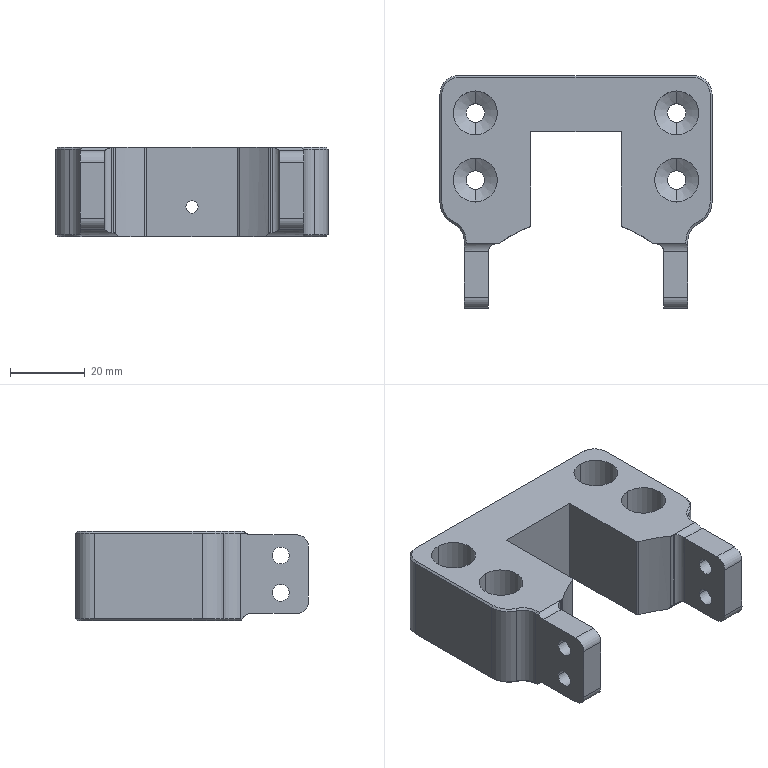NC program | NX | posted with a generic post | part box 73 x 62.4 x 24 mm
Lines 110 to 988 of 11507:
(ADAPTIVE_MILLING , TOOL : D10)
N176 T10 M6
N178 G54
N180 G17 G0 G90 X-47.247 Y-0.01 S8000 M3
N182 G43 Z30. H10
N184 Z-9.
N186 G94 G1 Z-12. F1000.
N188 X-45.053 Y-0.272 F3500.
N190 G3 X-44.622 Y-0.01 R0.536
N192 X-43.825 Y2.911 R7.188
N194 X-43.521 Y11.777 R90.492
N196 G1 X-43.514 Y13.652
N198 X-43.51 Y16.402
N200 X-43.508 Y21.652
N202 X-43.507 Y31.027
N204 X-43.506 Y31.277
N206 X-43.502 Y31.402
N208 G2 X-40.935 Y35.647 R5.829
N210 X-35.479 Y37.674 R12.556
N212 X-27.25 Y38.153 R59.855
N214 G1 X-26.25 Y38.162
N216 X-25.125 Y38.17
N218 X-23.5 Y38.177
N220 X-21.25 Y38.182
N222 X-17.625 Y38.185
N224 X-6. Y38.186
N226 X36.5
N228 X36.625 Y38.184
N230 X36.749 Y38.179
N232 X36.874 Y38.17
N234 G2 X41.05 Y35.485 R5.897
N236 X43.003 Y29.999 R12.841
N238 X43.452 Y22.018 R60.705
N240 G1 X43.463 Y20.893
N242 X43.471 Y19.518
N244 X43.478 Y17.643
N246 X43.482 Y15.268
N248 X43.485 Y10.768
N250 X43.486 Y-26.982
N252 Y-31.232
N254 X43.484 Y-31.357
N256 X43.477 Y-31.482
N258 X43.466 Y-31.606
N260 G2 X40.649 Y-35.837 R6.001
N262 X34.89 Y-37.759 R13.462
N264 X25.655 Y-38.167 R79.348
N266 G1 X24.155 Y-38.175
N268 X22.155 Y-38.18
N270 X19.03 Y-38.184
N272 X12.155 Y-38.186
N274 X-36.47
N276 X-36.595 Y-38.185
N278 G2 X-40.81 Y-35.809 R5.653
N280 X-42.96 Y-30.274 R12.12
N282 X-43.445 Y-22.546 R54.637
N284 X-43.457 Y-2.797 R922.246
N286 G3 X-42.766 Y4.168 R369.786
N288 X-42.523 Y17.914 R254.659
N290 G2 X-42.488 Y28.788 R700.753
N292 X-38.545 Y34.698 R7.841
N294 X-32.028 Y36.72 R16.354
N296 X-22.168 Y37.152 R90.427
N298 G1 X-20.793 Y37.16
N300 X-18.918 Y37.167
N302 X-16.293 Y37.172
N304 X-11.918 Y37.175
N306 X6.457
N308 X33.332
N310 G2 X39.797 Y33.54 R7.602
N312 X41.973 Y27.079 R15.41
N314 X42.447 Y17.472 R79.405
N316 G1 X42.457 Y16.097
N318 X42.464 Y14.472
N320 X42.469 Y12.347
N322 X42.473 Y8.847
N324 X42.475 Y1.097
N326 Y-28.028
N328 G2 X38.842 Y-34.494 R7.602
N330 X32.505 Y-36.656 R15.316
N332 X23.399 Y-37.141 R74.48
N334 G1 X22.274 Y-37.151
N336 X20.899 Y-37.16
N338 X19.274 Y-37.166
N340 X16.899 Y-37.171
N342 X13.024 Y-37.174
N344 X1.649 Y-37.175
N346 X-33.351
N348 X-33.601 Y-37.173
N350 X-33.851 Y-37.164
N352 G2 X-39.875 Y-33.42 R7.671
N354 X-41.991 Y-26.936 R15.797
N356 X-42.451 Y-16.953 R85.053
N358 X-42.428 Y-4.204 R448.54
N360 G3 X-41.769 Y4.771 R957.119
N362 G1 X-41.734 Y5.52
N364 X-41.703 Y6.27
N366 X-41.675 Y7.019
N368 X-41.651 Y7.769
N370 X-41.65 Y7.82
N372 Y26.186
N374 X-41.649 Y26.214
N376 X-41.458 Y28.153
N378 X-41.447 Y28.207
N380 X-40.885 Y30.058
N382 X-40.864 Y30.109
N384 X-39.952 Y31.815
N386 X-39.922 Y31.86
N388 X-38.695 Y33.356
N390 X-38.656 Y33.395
N392 X-37.16 Y34.622
N394 X-37.115 Y34.652
N396 X-35.409 Y35.564
N398 X-35.358 Y35.585
N400 X-33.507 Y36.147
N402 X-33.453 Y36.158
N404 X-31.514 Y36.349
N406 X-31.486 Y36.35
N408 X31.486
N410 X31.514 Y36.349
N412 X33.453 Y36.158
N414 X33.507 Y36.147
N416 X35.358 Y35.585
N418 X35.409 Y35.564
N420 X37.115 Y34.652
N422 X37.16 Y34.622
N424 X38.656 Y33.395
N426 X38.695 Y33.356
N428 X39.922 Y31.86
N430 X39.952 Y31.815
N432 X40.864 Y30.109
N434 X40.885 Y30.058
N436 X41.447 Y28.207
N438 X41.458 Y28.153
N440 X41.649 Y26.214
N442 X41.65 Y26.186
N444 Y-2.689
N446 X41.649 Y-2.711
N448 X41.629 Y-2.96
N450 G3 X41.488 Y-14.458 R298.961
N452 G2 X41.447 Y-26.458 R542.382
N454 X36.69 Y-33.65 R8.945
N456 X33.443 Y-34.995 R16.931
N458 X31.293 Y-36.18 R5.576
N460 G1 X30.018 Y-36.348
N462 X29.982 Y-36.35
N464 G2 X19.734 Y-36.22 R205.958
N466 G1 X18.734 Y-36.209
N468 X17.609 Y-36.201
N470 X16.109 Y-36.194
N472 X13.984 Y-36.189
N474 X10.359 Y-36.187
N476 X-3.516 Y-36.186
N478 X-4.266 Y-36.183
N480 X-5.391 Y-36.181
N482 X-6.266
N484 X-7.015 Y-36.179
N486 X-8.14
N488 X-8.515
N490 X-9.39 Y-36.177
N492 X-10.39 Y-36.178
N494 X-10.89 Y-36.179
N496 X-11.515 Y-36.177
N498 X-12.89 Y-36.178
N500 X-13.64 Y-36.179
N502 X-14.64 Y-36.176
N504 X-15.89 Y-36.178
N506 X-16.64 Y-36.176
N508 X-17.64 Y-36.177
N510 X-18.015 Y-36.178
N512 X-19.265 Y-36.175
N514 X-20.14 Y-36.176
N516 X-21.39 Y-36.174
N518 X-22.192 Y-36.176
N520 X-22.204 Y-36.179
N522 X-23.482 Y-36.348
N524 X-23.518 Y-36.35
N526 G2 X-31.142 Y-36.29 R145.108
N528 X-39.063 Y-31.222 R9.185
N530 X-41.041 Y-24.037 R19.418
N532 X-41.445 Y-13.049 R114.967
N534 X-41.405 Y-4.949 R285.925
N536 X-41.65 Y-2.689 R13.093
N538 G1 Y7.936
N540 G3 X-42.562 Y8.219 R0.5
N542 G1 X-42.912 Y7.71
N544 X-44.043 Y6.06 Z-11.9
N546 X-44.782 Y4.972
N548 X-44.832 Y4.754
N550 X-44.825 Y-16.153
N552 G3 X-44.01 Y-25.178 R60.801
N554 G1 X-43.51 Y-28.132
N556 G3 X-41.324 Y-33.684 R17.035
N558 X-38.292 Y-36.846 R11.782
N560 X-35.905 Y-38.261 R14.75
N562 G1 X-33.127 Y-39.557
N564 G3 X-32.683 Y-39.473 R0.513
N566 G1 X-31.648 Y-38.678
N568 X-30.063 Y-37.458 Z-12.
N570 X-29.852 Y-37.301
N572 X-29.665 Y-37.117
N574 G3 X-30.018 Y-36.348 R0.501
N576 G2 X-33.451 Y-35.106 R6.123
N578 X-39.075 Y-27.253 R13.64
N580 X-40.254 Y-19.107 R34.794
N582 X-40.454 Y-7.801 R296.213
N584 X-41.426 Y-4.863 R11.519
N586 G3 X-42.386 Y-4.822 R0.5
N588 G1 X-42.647 Y-5.603
N590 X-43.281 Y-7.499 Z-11.9
N592 X-43.669 Y-8.68
N594 X-43.679 Y-11.878
N596 X-43.649 Y-15.077
N598 G3 X-43.147 Y-21.853 R73.461
N600 G1 X-42.967 Y-23.333
N602 X-42.761 Y-24.81
N604 G3 X-41.089 Y-30.413 R22.619
N606 X-39.632 Y-33.007 R18.982
N608 X-36.901 Y-36.859 R63.987
N610 X-36.486 Y-36.999 R0.514
N612 G1 X-35.18 Y-36.831
N614 X-33.196 Y-36.575 Z-12.
N616 X-32.937 Y-36.546
N618 X-32.684 Y-36.481
N620 G3 X-32.604 Y-35.638 R0.501
N622 G2 X-34.505 Y-33.699 R5.992
N624 X-38.885 Y-21.875 R24.702
N626 X-39.417 Y-10.143 R111.218
N628 G3 X-39.498 Y-9.417 R5.368
N630 G2 X-40.455 Y-7.797 R15.222
N632 G3 X-41.388 Y-7.826 R0.501
N634 G1 X-41.457 Y-8.023
N636 X-42.117 Y-9.911 Z-11.9
N638 X-42.694 Y-11.573
N640 X-42.705 Y-11.694
N642 X-42.629 Y-14.189
N644 X-42.497 Y-16.681
N646 X-42.383 Y-17.923
N648 X-42.252 Y-19.163
N650 X-41.451 Y-25.67
N652 G3 X-39.988 Y-30.246 R15.486
N654 G1 X-38.741 Y-32.71
N656 X-38.653 Y-32.797
N658 X-38.551 Y-32.867
N660 X-37.31 Y-33.454
N662 X-35.502 Y-34.309 Z-12.
N664 X-35.005 Y-34.536
N666 G3 X-34.438 Y-33.804 R0.501
N668 G2 X-35.363 Y-31.177 R16.109
N670 X-38.205 Y-16.643 R45.398
N672 G3 X-38.447 Y-11.025 R192.609
N674 X-38.582 Y-10.529 R4.593
N676 G2 X-39.516 Y-9.388 R12.129
N678 G3 X-40.523 Y-9.784 R0.55
N680 G1 X-40.331 Y-10.77
N682 X-39.949 Y-12.733 Z-11.9
N684 X-37.652 Y-24.522
N686 X-37.27 Y-26.486 Z-12.
N688 X-36.04 Y-32.759
N690 G3 X-34.979 Y-32.496 R0.55
N692 G2 X-35.274 Y-29.689 R92.746
N694 X-36.6 Y-22.308 R220.445
N696 X-37.332 Y-13.091 R114.757
N698 G3 X-37.621 Y-11.5 R5.66
N700 G2 X-38.584 Y-10.527 R11.27
N702 G3 X-39.541 Y-10.977 R0.55
N704 G1 X-39.46 Y-11.469
N706 X-39.136 Y-13.442 Z-11.9
N708 X-37.651 Y-22.462
N710 X-37.327 Y-24.435 Z-12.
N712 X-36.221 Y-31.109
N714 G3 X-35.15 Y-30.932 R0.55
N716 X-35.615 Y-22.33 R51.445
N718 G2 X-36.317 Y-13.859 R506.421
N720 G3 X-36.68 Y-12.283 R6.352
N722 G1 X-36.755 Y-12.19
N724 X-37.716 Y-11.387
N726 G3 X-38.612 Y-11.892 R0.551
N728 G1 X-36.244 Y-27.39
N730 G3 X-35.15 Y-27.307 R0.55
N732 X-35.19 Y-16.557 R427.104
N734 X-35.739 Y-12.99 R11.724
N736 G1 X-35.962 Y-12.666
N738 X-36.72 Y-12.214
N740 X-36.757 Y-12.188
N742 G3 X-37.605 Y-12.782 R0.551
N744 G1 X-36.201 Y-17.909
N746 G3 X-35.15 Y-17.682 R0.55
N748 X-35.19 Y-13.559 R55.738
N750 X-35.474 Y-12.957 R1.065
N752 G1 X-36.011 Y-12.637
N754 G3 X-36.738 Y-13.431 R0.55
N756 G1 X-36.09 Y-14.319
N758 G3 X-35.15 Y-13.932 R0.551
N760 X-35.278 Y-13.112 R1.289
N762 G1 X-35.425 Y-12.986
N764 X-35.532 Y-12.922
N766 G3 X-36.163 Y-13.021 R0.504
N768 G1 X-36.323 Y-13.203
N770 X-37.646 Y-14.703 Z-11.9
N772 X-38.633 Y-15.831
N774 X-38.69 Y-15.963
N776 X-38.714 Y-16.104
N778 X-38.707 Y-29.055
N780 G3 X-37.508 Y-34.639 R16.449
N782 X-35.731 Y-37.093 R7.053
N784 G1 X-34.606 Y-38.082
N786 G3 X-32.584 Y-38.971 R4.306
N788 X-29.225 Y-39.383 R37.795
N790 G1 X-27.623 Y-39.436
N792 X20.376 Y-39.524
N794 X20.485 Y-39.488
N796 X20.588 Y-39.439
N798 X21.723 Y-38.643
N800 X23.36 Y-37.494 Z-12.
N802 X23.769 Y-37.198
N804 G3 X23.482 Y-36.348 R0.501
N806 G2 X21.308 Y-35.87 R6.827
N808 G3 X15.6 Y-35.283 R27.258
N810 X-4.149 Y-35.186 R984.653
N812 G1 X-5.274 Y-35.184
N814 X-6.149
N816 X-7.149 Y-35.181
N818 X-8.274 Y-35.182
N820 X-9.024 Y-35.18
N822 X-10.149
N824 X-10.774 Y-35.181
N826 X-12.024 Y-35.177
N828 X-13.024 Y-35.179
N830 X-14.149 Y-35.177
N832 X-15.149 Y-35.178
N834 X-16.149 Y-35.176
N836 X-16.899
N838 X-17.649 Y-35.178
N840 X-18.774 Y-35.175
N842 X-19.524 Y-35.176
N844 X-19.649 Y-35.177
N846 X-19.899 Y-35.181
N848 G3 X-20.415 Y-35.269 R1.866
N850 G1 X-20.896 Y-35.638
N852 X-20.959 Y-35.674
N854 X-22.133 Y-36.16
N856 X-22.204 Y-36.179
N858 G3 X-22.06 Y-37.261 R0.55
N860 G1 X-20.92 Y-37.257
N862 X-18.92 Y-37.251 Z-11.9
N864 X18.72 Y-37.132
N866 X20.72 Y-37.126 Z-12.
N868 X21.782 Y-37.115
N870 G3 X21.902 Y-36.065 R0.55
N872 G2 X19.994 Y-35.21 R91.635
N874 G3 X14.574 Y-34.382 R20.379
N876 X-0.673 Y-34.201 R389.778
N878 G1 X-1.423 Y-34.197
N880 X-2.548 Y-34.194
N882 X-3.548 Y-34.193
N884 X-4.423 Y-34.189
N886 X-5.298 Y-34.188
N888 X-6.173 Y-34.186
N890 X-6.798 Y-34.183
N892 X-7.923 Y-34.184
N894 X-8.548 Y-34.182
N896 X-9.173 Y-34.18
N898 X-10.173 Y-34.181
N900 X-11.298 Y-34.178
N902 X-12.548 Y-34.18
N904 X-13.798 Y-34.177
N906 X-14.798 Y-34.179
N908 X-15.798 Y-34.176
N910 G3 X-19.289 Y-34.322 R20.036
N912 X-19.888 Y-34.864 R1.346
N914 G1 X-20.483 Y-35.321
N916 G3 X-20.152 Y-36.307 R0.551
N918 G1 X-19.86 Y-36.309
N920 X-17.86 Y-36.325 Z-11.9
N922 X18.083 Y-36.605
N924 X20.083 Y-36.62 Z-12.
N926 X20.648 Y-36.617
N928 G3 X20.896 Y-35.638 R0.551
N930 X17.074 Y-33.911 R7.517
N932 X9.608 Y-33.3 R45.798
N934 X-12.141 Y-33.18 R985.897
N936 X-17.762 Y-33.296 R58.939
N938 X-18.946 Y-33.652 R2.657
N940 G1 X-19.026 Y-33.741
N942 X-19.062 Y-33.804
N944 X-19.595 Y-34.498
N946 G3 X-19.173 Y-35.383 R0.551
N948 G1 X-17.173 Y-35.416 Z-11.9
N950 X17.573 Y-35.98
N952 X19.572 Y-36.012 Z-12.
N954 G3 X20.082 Y-35.916 R0.788
N956 X20.102 Y-35.029 R0.551
N958 X19.195 Y-34.223 R26.233
N960 X15.075 Y-32.848 R10.727
N962 X6.475 Y-32.29 R63.923
N964 X-15.399 Y-32.225 R858.486
N966 X-18.333 Y-32.75 R7.91
N968 X-18.752 Y-33.08 R1.363
N970 G1 X-19.026 Y-33.741
N972 X-19.062 Y-33.804
N974 G3 X-18.719 Y-34.613 R0.551
N976 G1 X-18.066 Y-34.649 Z-11.967
N978 X-17.413 Y-34.659 Z-11.935
N980 X-16.721 Y-34.677 Z-11.9
N982 X17.237 Y-35.545
N984 X19.236 Y-35.596 Z-12.
N986 G3 X19.76 Y-34.713 R0.555
N988 X16.763 Y-32.587 R5.404
N990 X10.121 Y-31.496 R25.906
N992 X-7.249 Y-31.198 R351.051
N994 X-15.371 Y-31.319 R108.78
N996 X-18.241 Y-32.096 R6.684
N998 X-18.54 Y-32.567 R0.772
N1000 G1 X-18.779 Y-33.144
N1002 G3 X-18.424 Y-33.883 R0.552
N1004 G1 X-18.014 Y-33.918 Z-11.979
N1006 X-17.602 Y-33.925 Z-11.959
N1008 X-16.427 Y-33.96 Z-11.9
N1010 X16.833 Y-34.943
N1012 X18.832 Y-35.002 Z-12.
N1014 G3 X19.303 Y-34.118 R0.551
N1016 X16.439 Y-31.868 R5.313
N1018 X10.085 Y-30.609 R23.042
N1020 X-2.657 Y-30.232 R190.371
N1022 X-13.905 Y-30.297 R198.112
N1024 X-17.666 Y-31.119 R10.073
N1026 X-18.433 Y-31.833 R1.481
N1028 G1 X-18.515 Y-32.453
N1030 G3 X-18.117 Y-33.055 R0.554
N1032 G1 X-17.562 Y-33.097 Z-11.972
N1034 X-17.006 Y-33.113 Z-11.944
N1036 X-16.12 Y-33.147 Z-11.9
N1038 X16.6 Y-34.427
N1040 X17.599 Y-34.471 Z-11.95
N1042 X18.598 Y-34.495 Z-12.
N1044 G3 X19.026 Y-33.741 R0.552
N1046 X17.051 Y-31.579 R3.963
N1048 X11.575 Y-29.931 R15.88
N1050 X1.226 Y-29.304 R86.142
N1052 X-12.398 Y-29.282 R288.85
N1054 X-17.049 Y-30.119 R13.975
N1056 X-18.322 Y-31.077 R2.391
N1058 G1 X-18.35 Y-31.174
N1060 X-18.352 Y-31.218
N1062 X-18.434 Y-31.838
N1064 G3 X-18.014 Y-32.445 R0.554
N1066 G1 X-17.016 Y-32.503 Z-11.95
N1068 X-16.017 Y-32.542 Z-11.9
N1070 X16.401 Y-33.956
N1072 X18.399 Y-34.035 Z-12.
N1074 G3 X18.835 Y-33.279 R0.551
N1076 X16.57 Y-30.731 R4.432
N1078 X10.984 Y-29.012 R16.632
N1080 X0.764 Y-28.329 R80.747
N1082 X-11.858 Y-28.322 R203.986
N1084 X-16.862 Y-29.294 R14.608
N1086 X-18.315 Y-30.427 R2.941
N1088 X-18.35 Y-31.182 R6.511
N1090 X-17.918 Y-31.719 R0.554
N1092 G1 X-15.921 Y-31.817 Z-11.9
N1094 X16.131 Y-33.261
N1096 X18.072 Y-33.346 Z-11.997
N1098 X18.129 Y-33.339 Z-12.
N1100 G3 X18.548 Y-32.586 R0.552
N1102 X17.107 Y-30.506 R3.416
N1104 X12.072 Y-28.4 R12.853
N1106 X2.51 Y-27.422 R54.422
N1108 X-11.236 Y-27.352 R182.619
N1110 X-16.717 Y-28.469 R15.556
N1112 X-18.286 Y-29.668 R3.76
N1114 X-18.35 Y-30.623 R2.662
N1116 X-17.862 Y-31.169 R0.554
N1118 G1 X-15.865 Y-31.272 Z-11.9
N1120 X16.053 Y-32.898
N1122 X17.991 Y-32.993 Z-11.997
N1124 X18.05 Y-32.987 Z-12.
N1126 G3 X18.504 Y-32.372 R0.553
N1128 X17.133 Y-29.941 R3.434
N1130 X12.194 Y-27.63 R12.185
N1132 X2.779 Y-26.486 R47.486
N1134 X-10.716 Y-26.389 R153.661
N1136 X-16.327 Y-27.513 R17.265
N1138 X-18.304 Y-28.981 R4.259
N1140 X-18.35 Y-29.892 R3.558
N1142 X-17.855 Y-30.439 R0.554
N1144 G1 X-15.859 Y-30.554 Z-11.9
N1146 X15.982 Y-32.389
N1148 X17.921 Y-32.498 Z-11.997
N1150 X17.979 Y-32.492 Z-12.
N1152 G3 X18.439 Y-31.877 R0.553
N1154 X16.996 Y-29.208 R3.724
N1156 X12.099 Y-26.808 R12.343
N1158 X3.201 Y-25.568 R43.237
N1160 X-10.042 Y-25.42 R129.589
N1162 X-16.142 Y-26.635 R18.703
N1164 X-18.26 Y-28.136 R5.105
N1166 G1 X-18.314 Y-28.249
N1168 X-18.346 Y-28.37
N1170 X-18.35 Y-28.389
N1172 Y-29.264
N1174 G3 X-17.855 Y-29.811 R0.554
N1176 G1 X-15.859 Y-29.927 Z-11.9
N1178 X15.896 Y-31.769
N1180 X17.837 Y-31.878 Z-11.997
N1182 X17.893 Y-31.873 Z-12.
N1184 G3 X18.358 Y-31.257 R0.553
N1186 X17.291 Y-28.855 R3.366
N1188 X12.684 Y-26.191 R11.103
N1190 X4.333 Y-24.717 R35.866
N1192 X-9.531 Y-24.462 R112.459
N1194 X-15.995 Y-25.76 R19.694
N1196 X-18.291 Y-27.424 R5.073
N1198 X-18.35 Y-28.49 R3.272
N1200 X-17.854 Y-29.038 R0.554
N1202 G1 X-15.859 Y-29.175 Z-11.9
N1204 X15.853 Y-31.349
N1206 X17.848 Y-31.479 Z-12.
N1208 G3 X18.35 Y-30.932 R0.554
N1210 X17.312 Y-28.214 R3.499
N1212 X12.776 Y-25.429 R11.162
N1214 X4.33 Y-23.799 R34.236
N1216 X-9.654 Y-23.549 R94.121
N1218 X-16.089 Y-24.981 R19.314
N1220 X-18.275 Y-26.597 R5.323
N1222 X-18.35 Y-27.706 R2.906
N1224 X-17.853 Y-28.253 R0.554
N1226 G1 X-15.859 Y-28.399 Z-11.9
N1228 X15.844 Y-30.715
N1230 X17.839 Y-30.855 Z-12.
N1232 G3 X18.35 Y-30.307 R0.553
N1234 X17.184 Y-27.383 R3.742
N1236 X12.416 Y-24.498 R11.946
N1238 X3.849 Y-22.837 R35.21
N1240 X-9.759 Y-22.641 R81.005
N1242 X-16.278 Y-24.243 R18.698
N1244 X-18.305 Y-25.856 R4.813
N1246 X-18.35 Y-26.89 R4.216
N1248 X-17.852 Y-27.437 R0.554
N1250 G1 X-15.858 Y-27.594 Z-11.9
N1252 X15.844 Y-30.08
N1254 X17.838 Y-30.23 Z-12.
N1256 G3 X18.35 Y-29.682 R0.553
N1258 X17.236 Y-26.731 R3.842
N1260 X12.541 Y-23.732 R11.816
N1262 X3.879 Y-21.917 R34.619
N1264 X-9.724 Y-21.727 R72.824
N1266 X-16.231 Y-23.384 R19.034
N1268 X-18.278 Y-24.984 R5.434
N1270 X-18.35 Y-26.083 R2.96
N1272 X-17.851 Y-26.63 R0.554
N1274 G1 X-15.858 Y-26.797 Z-11.9
N1276 X15.844 Y-29.445
N1278 X17.837 Y-29.605 Z-12.
N1280 G3 X18.35 Y-29.057 R0.553
N1282 X17.223 Y-25.983 R3.972
N1284 X12.331 Y-22.834 R12.176
N1286 X3.429 Y-20.954 R34.889
N1288 X-9.798 Y-20.828 R65.326
N1290 X-16.281 Y-22.572 R18.915
N1292 X-18.298 Y-24.204 R5.104
N1294 X-18.35 Y-25.254 R3.594
N1296 X-17.851 Y-25.802 R0.554
N1298 G1 X-15.858 Y-25.973 Z-11.9
N1300 X15.844 Y-28.691
N1302 X17.837 Y-28.855 Z-12.
N1304 G3 X18.35 Y-28.307 R0.553
N1306 X17.135 Y-25.135 R4.141
N1308 X12.129 Y-21.93 R12.719
N1310 X2.861 Y-19.977 R36.117
N1312 X-10.113 Y-19.961 R58.982
N1314 X-16.546 Y-21.87 R18.124
N1316 X-18.315 Y-23.411 R4.558
N1318 X-18.35 Y-24.423 R7.125
N1320 X-17.85 Y-24.971 R0.554
N1322 G1 X-15.858 Y-25.153 Z-11.9
N1324 X15.844 Y-28.055
N1326 X17.836 Y-28.23 Z-12.
N1328 G3 X18.35 Y-27.682 R0.553
N1330 X17.143 Y-24.379 R4.248
N1332 X12.174 Y-21.115 R12.813
N1334 X2.929 Y-19.062 R35.432
N1336 X-10.289 Y-19.088 R55.082
N1338 X-16.689 Y-21.101 R17.641
N1340 X-18.326 Y-22.601 R4.094
N1342 G1 X-18.35 Y-22.707
N1344 Y-23.582
N1346 G3 X-17.849 Y-24.129 R0.554
N1348 G1 X-15.858 Y-24.317 Z-11.9
N1350 X15.844 Y-27.3
N1352 X17.835 Y-27.48 Z-12.
N1354 G3 X18.35 Y-26.932 R0.553
N1356 X17.157 Y-23.621 R4.303
N1358 X11.994 Y-20.205 R13.106
N1360 X2.505 Y-18.099 R35.863
N1362 X-10.706 Y-18.255 R50.581
N1364 X-16.823 Y-20.332 R17.02
N1366 X-18.292 Y-21.664 R4.713
N1368 X-18.35 Y-22.728 R3.321
N1370 X-17.849 Y-23.276 R0.554
N1372 G1 X-15.858 Y-23.469 Z-11.9
N1374 X15.843 Y-26.544
N1376 X17.834 Y-26.731 Z-12.
N1378 G3 X18.35 Y-26.182 R0.553
N1380 X17.097 Y-22.764 R4.443
N1382 X11.822 Y-19.29 R13.528
N1384 X1.966 Y-17.12 R36.797
N1386 X-10.498 Y-17.323 R48.921
N1388 X-16.847 Y-19.487 R17.513
N1390 X-18.302 Y-20.833 R4.571
N1392 X-18.35 Y-21.875 R3.852
N1394 X-17.848 Y-22.423 R0.554
N1396 G1 X-15.858 Y-22.622 Z-11.9
N1398 X15.843 Y-25.789
N1400 X17.834 Y-25.981 Z-12.
N1402 G3 X18.35 Y-25.432 R0.553
N1404 X17.045 Y-21.906 R4.552
N1406 X11.891 Y-18.468 R13.684
N1408 X1.433 Y-16.151 R36.745
N1410 X-10.899 Y-16.501 R45.673
N1412 X-16.968 Y-18.708 R16.642
N1414 X-18.309 Y-19.995 R4.35
N1416 X-18.35 Y-21.02 R4.788
N1418 X-17.847 Y-21.568 R0.554
N1420 G1 X-15.858 Y-21.773 Z-11.9
N1422 X15.843 Y-25.033
N1424 X17.833 Y-25.231 Z-12.
N1426 G3 X18.35 Y-24.682 R0.553
N1428 X17.083 Y-21.141 R4.562
N1430 X11.736 Y-17.55 R13.932
N1432 X0.908 Y-15.185 R37.156
N1434 X-11.413 Y-15.71 R43.248
N1436 X-17.186 Y-17.994 R15.571
N1438 X-18.312 Y-19.146 R4.039
N1440 X-18.35 Y-20.164 R5.761
N1442 X-17.848 Y-20.712 R0.554
N1444 G1 X-15.858 Y-20.915 Z-11.9
N1446 X15.843 Y-24.159
N1448 X17.833 Y-24.356 Z-12.
N1450 G3 X18.35 Y-23.807 R0.553
N1452 X17.123 Y-20.373 R4.571
N1454 X12.046 Y-16.823 R13.691
N1456 X1.382 Y-14.312 R35.385
N1458 X-11.311 Y-14.798 R42.731
N1460 X-13.157 Y-15.29 R19.309
N1462 X-18.123 Y-18.343 R30.86
N1464 X-18.35 Y-18.767 R1.056
N1466 G1 Y-19.392
N1468 G3 X-17.288 Y-19.593 R0.55
N1470 G1 X-16.912 Y-18.612
N1472 G3 X-17.736 Y-18.029 R0.551
N1474 X-18.35 Y-18.719 R0.914
N1476 G1 Y-18.844
N1478 G3 X-17.865 Y-19.39 R0.554
N1480 G1 X-17.653 Y-19.415
N1482 X-15.667 Y-19.65 Z-11.9
N1484 X15.843 Y-23.379
N1486 X17.83 Y-23.606 Z-12.
N1488 G3 X18.35 Y-23.057 R0.553
N1490 X17.167 Y-19.607 R4.588
N1492 X12.016 Y-15.95 R13.724
N1494 X1.737 Y-13.43 R34.868
N1496 X-9.553 Y-13.593 R44.537
N1498 G2 X-13.091 Y-15.259 R31.444
N1500 G3 X-12.984 Y-16.302 R0.55
N1502 G1 X-12.417 Y-16.421
N1504 X-10.459 Y-16.83 Z-11.9
N1506 X15.836 Y-22.333
N1508 X17.741 Y-22.728 Z-11.997
N1510 X17.795 Y-22.732 Z-12.
N1512 G3 X18.35 Y-22.182 R0.553
N1514 X17.139 Y-18.74 R4.632
N1516 X11.877 Y-15.023 R14.076
N1518 X0.976 Y-12.443 R35.475
N1520 X-8.253 Y-12.546 R38.892
N1522 G1 X-8.37 Y-12.588
N1524 X-8.478 Y-12.649
N1526 G2 X-9.575 Y-13.605 R9.49
N1528 G3 X-9.454 Y-14.622 R0.551
N1530 G1 X-7.524 Y-15.144 Z-11.9
N1532 X15.832 Y-21.468
N1534 X17.71 Y-21.974 Z-11.997
N1536 X17.765 Y-21.98 Z-12.
N1538 G3 X18.35 Y-21.432 R0.552
N1540 X17.117 Y-17.872 R4.717
N1542 G1 X17.037 Y-17.776
N1544 X16.956 Y-17.681
N1546 X16.873 Y-17.587
N1548 X16.79 Y-17.494
N1550 X16.705 Y-17.402
N1552 X16.607 Y-17.299
N1554 G3 X10.778 Y-14.251 R30.356
N1556 X4.196 Y-11.988 R19.033
N1558 X-6.883 Y-11.515 R39.216
N1560 X-7.921 Y-11.9 R1.849
N1562 G2 X-8.513 Y-12.681 R3.388
N1564 G3 X-8.378 Y-13.582 R0.551
N1566 G1 X-6.459 Y-14.143 Z-11.9
N1568 X15.837 Y-20.564
N1570 X17.704 Y-21.098 Z-11.997
N1572 X17.762 Y-21.105 Z-12.
N1574 G3 X18.35 Y-20.557 R0.552
N1576 X17.846 Y-18.15 R4.163
N1578 X16.503 Y-17.231 R21.091
N1580 X15.762 Y-18.022 R0.55
N1582 G1 X17.422 Y-20.206
N1584 G3 X18.35 Y-19.807 R0.551
N1586 X18.243 Y-18.447 R3.756
N1588 X17.711 Y-18.025 R1.663
N1590 X16.995 Y-18.847 R0.55
N1592 G1 X17.45 Y-19.356
N1594 G3 X18.35 Y-18.932 R0.551
N1596 X18.117 Y-18.288 R0.689
N1598 G1 X9.677 Y-13.66
N1600 G2 X8.748 Y-12.932 R6.032
N1602 G3 X4.35 Y-11.218 R12.382
N1604 X-5.839 Y-10.565 R33.416
N1606 X-7.369 Y-11.052 R3.117
N1608 G1 X-7.448 Y-11.152
N1610 X-7.454 Y-11.167
N1612 X-7.483 Y-11.227
N1614 X-7.96 Y-11.961
N1616 G3 X-7.641 Y-12.792 R0.551
N1618 G1 X-5.649 Y-12.962 Z-11.9
N1620 X6.26 Y-13.928
N1622 X8.253 Y-14.09 Z-12.
N1624 X8.528 Y-14.116
N1626 X8.804 Y-14.104
N1628 G3 X9.04 Y-13.167 R0.551
N1630 X7.311 Y-11.68 R11.912
N1632 X1.987 Y-9.968 R15.286
N1634 X-5.358 Y-9.711 R25.42
N1636 X-7.101 Y-10.343 R3.92
N1638 X-7.454 Y-11.167 R2.646
N1640 X-7.131 Y-11.864 R0.553
N1642 G1 X-6.77 Y-11.924 Z-11.982
N1644 X-6.405 Y-11.953 Z-11.963
N1646 X-5.144 Y-12.073 Z-11.9
N1648 X5.715 Y-13.11
N1650 X7.706 Y-13.3 Z-12.
N1652 G3 X8.284 Y-12.459 R0.554
N1654 X5.639 Y-10.265 R5.28
N1656 X-4.902 Y-8.87 R21.261
N1658 X-6.955 Y-9.707 R3.909
N1660 X-7.257 Y-10.607 R17.87
N1662 X-6.934 Y-11.304 R0.553
N1664 G1 X-6.574 Y-11.365 Z-11.982
N1666 X-6.211 Y-11.396 Z-11.963
N1668 X-4.948 Y-11.525 Z-11.9
N1670 X5.364 Y-12.572
N1672 X7.354 Y-12.774 Z-12.
N1674 G3 X7.943 Y-11.935 R0.555
N1676 X4.791 Y-9.264 R5.948
N1678 X-4.647 Y-8.08 R18.146
N1680 X-6.885 Y-9.098 R4.024
N1682 X-7.063 Y-9.95 R2.003
N1684 X-6.674 Y-10.539 R0.554
N1686 G1 X-5.682 Y-10.659 Z-11.95
N1688 X-4.688 Y-10.762 Z-11.9
N1690 X5.027 Y-11.811
N1692 X7.016 Y-12.019 Z-12.
N1694 G3 X7.483 Y-11.227 R0.551
N1696 X5.583 Y-9.064 R4.149
N1698 X-1.081 Y-7.138 R14.985
N1700 X-5.753 Y-7.716 R10.261
N1702 X-6.914 Y-8.619 R2.259
N1704 G1 X-6.946 Y-8.74
N1706 X-6.95 Y-8.759
N1708 Y-8.938
N1710 X-6.952 Y-8.97
N1712 X-6.994 Y-9.343
N1714 G3 X-6.568 Y-9.941 R0.554
N1716 G1 X-4.585 Y-10.199 Z-11.9
N1718 X4.885 Y-11.416
N1720 X6.87 Y-11.664 Z-12.
N1722 G3 X7.371 Y-10.932 R0.551
N1724 X5.254 Y-8.259 R4.431
N1726 X-4.507 Y-6.609 R13.882
N1728 X-6.796 Y-7.81 R4.364
N1730 G1 X-6.869 Y-7.912
N1732 X-6.919 Y-8.026
N1734 X-6.95 Y-8.153
N1736 Y-8.778
N1738 G3 X-6.497 Y-9.32 R0.554
N1740 G1 X-4.513 Y-9.569 Z-11.9
N1742 X4.652 Y-10.717
N1744 X5.644 Y-10.846 Z-11.95
N1746 X6.637 Y-10.956 Z-12.
N1748 G3 X7.122 Y-10.224 R0.551
N1750 X5.554 Y-7.866 R3.723
N1752 X-1.099 Y-5.607 R12.286
N1754 X-5.955 Y-6.485 R8.92
N1756 X-6.929 Y-7.419 R2.148
N1758 G1 X-6.95 Y-7.511
N1760 Y-8.261
N1762 G3 X-6.447 Y-8.81 R0.555
N1764 G1 X-4.465 Y-9.078 Z-11.9
N1766 X4.586 Y-10.305
N1768 X6.506 Y-10.562 Z-11.997
N1770 X6.569 Y-10.559 Z-12.
N1772 G3 X7.063 Y-9.95 R0.553
N1774 X5.699 Y-7.379 R3.545
N1776 X-0.351 Y-4.93 R11.11
N1778 X-5.723 Y-5.683 R9.505
N1780 X-6.922 Y-6.738 R2.611
N1782 G1 X-6.95 Y-6.86
N1784 Y-7.61
N1786 G3 X-6.436 Y-8.161 R0.557
N1788 G1 X-4.457 Y-8.454 Z-11.9
N1790 X4.524 Y-9.784
N1792 X6.441 Y-10.065 Z-11.997
N1794 X6.504 Y-10.063 Z-12.
N1796 G3 X7.007 Y-9.453 R0.552
N1798 X5.567 Y-6.632 R3.779
N1800 X-0.852 Y-4.152 R10.926
N1802 X-5.934 Y-5.12 R8.871
N1804 X-6.918 Y-6.052 R2.564
N1806 X-6.95 Y-6.932 R13.436
N1808 X-6.433 Y-7.484 R0.558
N1810 G1 X-4.457 Y-7.793 Z-11.9
N1812 X4.458 Y-9.191
N1814 X6.375 Y-9.488 Z-11.997
N1816 X6.435 Y-9.487 Z-12.
N1818 G3 X6.95 Y-8.938 R0.553
N1820 X5.845 Y-6.253 R3.414
N1822 X0.067 Y-3.53 R10.059
N1824 X-5.668 Y-4.281 R9.586
N1826 X-6.897 Y-5.315 R3.299
N1828 X-6.95 Y-6.243 R3.019
N1830 X-6.428 Y-6.797 R0.56
N1832 G1 X-4.457 Y-7.135 Z-11.9
N1834 X4.445 Y-8.661
N1836 X6.362 Y-8.987 Z-11.997
N1838 X6.417 Y-8.988 Z-12.
N1840 G3 X6.95 Y-8.438 R0.553
N1842 X5.784 Y-5.521 R3.629
N1844 X-0.367 Y-2.759 R10.07
N1846 X-5.828 Y-3.678 R9.192
N1848 X-6.917 Y-4.678 R2.769
N1850 X-6.95 Y-5.56 R9.677
N1852 X-6.427 Y-6.114 R0.561
N1854 G1 X-4.457 Y-6.461 Z-11.9
N1856 X4.445 Y-8.028
N1858 X6.36 Y-8.362 Z-11.997
N1860 X6.416 Y-8.363 Z-12.
N1862 G3 X6.95 Y-7.813 R0.553
N1864 X5.733 Y-4.785 R3.779
N1866 X-0.673 Y-2.018 R10.063
N1868 X-5.98 Y-3.078 R8.818
N1870 X-6.932 Y-4.037 R2.24
N1872 G1 X-6.95 Y-4.118
N1874 Y-4.868
N1876 G3 X-6.425 Y-5.423 R0.563
N1878 G1 X-4.457 Y-5.779 Z-11.9
N1880 X4.445 Y-7.393
N1882 X6.358 Y-7.737 Z-11.997
N1884 X6.414 Y-7.738 Z-12.
N1886 G3 X6.95 Y-7.188 R0.553
N1888 X5.689 Y-4.052 R3.85
N1890 X-0.848 Y-1.294 R10.05
N1892 X-6.019 Y-2.407 R8.705
N1894 X-6.943 Y-3.387 R1.976
N1896 G1 X-6.95 Y-3.419
N1898 Y-4.169
N1900 G3 X-6.423 Y-4.724 R0.565
N1902 G1 X-4.457 Y-5.092 Z-11.9
N1904 X4.445 Y-6.757
N1906 X6.355 Y-7.112 Z-11.997
N1908 X6.412 Y-7.113 Z-12.
N1910 G3 X6.95 Y-6.563 R0.553
N1912 X5.65 Y-3.315 R3.938
N1914 X-1.147 Y-0.574 R10.069
N1916 X-6.162 Y-1.806 R8.4
N1918 X-6.95 Y-2.736 R1.679
N1920 G1 Y-3.486
N1922 G3 X-6.424 Y-4.04 R0.563
N1924 G1 X-4.457 Y-4.398 Z-11.9
N1926 X4.445 Y-6.017